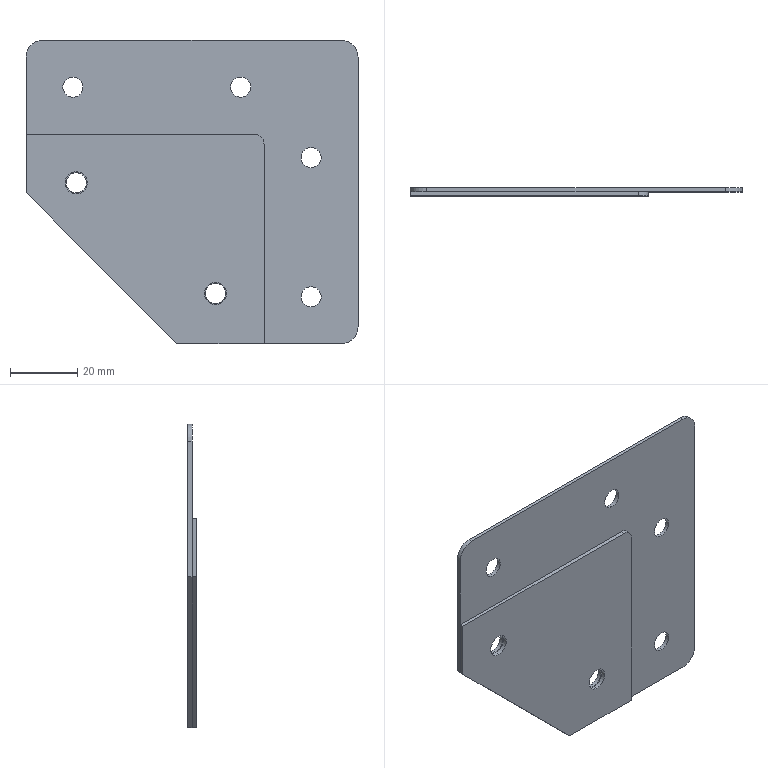Part | SolidWorks | features ICE 9, EdgeFlange 2, Fillet 2, HoleWzd 2, FlatPattern 1, SMBaseFlange 1, SheetMetal 1, WeldmentFeature 1 | 2 solids | 34 faces | box 99 x 2.4 x 90.5 mm | volume 13339 mm3 | cylinder 20 | plane 14 | commonest cylinder face diameters 6 x13 6.6 x4 10 x3
STEP:
#1=CARTESIAN_POINT('',(553.,-1.2,256.7));
#2=VERTEX_POINT('',#1);
#3=CARTESIAN_POINT('',(553.,-1.2,263.3));
#4=VERTEX_POINT('',#3);
#5=CARTESIAN_POINT('',(553.,-1.2,260.));
#6=DIRECTION('',(0.,1.,0.));
#7=DIRECTION('',(0.,0.,1.));
#8=AXIS2_PLACEMENT_3D('',#5,#6,#7);
#9=CIRCLE('',#8,3.3);
#10=EDGE_CURVE('',#2,#4,#9,.T.);
#11=ORIENTED_EDGE('',*,*,#10,.F.);
#12=CARTESIAN_POINT('',(553.,0.,256.7));
#13=VERTEX_POINT('',#12);
#14=CARTESIAN_POINT('',(553.,0.,256.7));
#15=DIRECTION('',(0.,1.,0.));
#16=VECTOR('',#15,1000.);
#17=LINE('',#14,#16);
#18=EDGE_CURVE('',#2,#13,#17,.T.);
#19=ORIENTED_EDGE('',*,*,#18,.T.);
#20=CARTESIAN_POINT('',(553.,0.,263.3));
#21=VERTEX_POINT('',#20);
#22=CARTESIAN_POINT('',(553.,0.,260.));
#23=DIRECTION('',(0.,1.,0.));
#24=DIRECTION('',(0.,0.,1.));
#25=AXIS2_PLACEMENT_3D('',#22,#23,#24);
#26=CIRCLE('',#25,3.3);
#27=EDGE_CURVE('',#13,#21,#26,.T.);
#28=ORIENTED_EDGE('',*,*,#27,.T.);
#29=CARTESIAN_POINT('',(553.,0.,263.3));
#30=DIRECTION('',(0.,1.,0.));
#31=VECTOR('',#30,1000.);
#32=LINE('',#29,#31);
#33=EDGE_CURVE('',#4,#21,#32,.T.);
#34=ORIENTED_EDGE('',*,*,#33,.F.);
#35=EDGE_LOOP('',(#11,#19,#28,#34));
#36=FACE_OUTER_BOUND('',#35,.T.);
#37=CARTESIAN_POINT('',(553.,0.,260.));
#38=DIRECTION('',(0.,1.,0.));
#39=DIRECTION('',(0.,0.,1.));
#40=AXIS2_PLACEMENT_3D('',#37,#38,#39);
#41=CYLINDRICAL_SURFACE('',#40,3.3);
#42=ADVANCED_FACE('',(#36),#41,.F.);
#43=CARTESIAN_POINT('',(511.5,-1.2,289.7));
#44=VERTEX_POINT('',#43);
#45=CARTESIAN_POINT('',(511.5,-1.2,296.3));
#46=VERTEX_POINT('',#45);
#47=CARTESIAN_POINT('',(511.5,-1.2,293.));
#48=DIRECTION('',(0.,1.,0.));
#49=DIRECTION('',(0.,0.,1.));
#50=AXIS2_PLACEMENT_3D('',#47,#48,#49);
#51=CIRCLE('',#50,3.3);
#52=EDGE_CURVE('',#44,#46,#51,.T.);
#53=ORIENTED_EDGE('',*,*,#52,.F.);
#54=CARTESIAN_POINT('',(511.5,0.,289.7));
#55=VERTEX_POINT('',#54);
#56=CARTESIAN_POINT('',(511.5,0.,289.7));
#57=DIRECTION('',(0.,1.,0.));
#58=VECTOR('',#57,1000.);
#59=LINE('',#56,#58);
#60=EDGE_CURVE('',#44,#55,#59,.T.);
#61=ORIENTED_EDGE('',*,*,#60,.T.);
#62=CARTESIAN_POINT('',(511.5,0.,296.3));
#63=VERTEX_POINT('',#62);
#64=CARTESIAN_POINT('',(511.5,0.,293.));
#65=DIRECTION('',(0.,1.,0.));
#66=DIRECTION('',(0.,0.,1.));
#67=AXIS2_PLACEMENT_3D('',#64,#65,#66);
#68=CIRCLE('',#67,3.3);
#69=EDGE_CURVE('',#55,#63,#68,.T.);
#70=ORIENTED_EDGE('',*,*,#69,.T.);
#71=CARTESIAN_POINT('',(511.5,0.,296.3));
#72=DIRECTION('',(0.,1.,0.));
#73=VECTOR('',#72,1000.);
#74=LINE('',#71,#73);
#75=EDGE_CURVE('',#46,#63,#74,.T.);
#76=ORIENTED_EDGE('',*,*,#75,.F.);
#77=EDGE_LOOP('',(#53,#61,#70,#76));
#78=FACE_OUTER_BOUND('',#77,.T.);
#79=CARTESIAN_POINT('',(511.5,0.,293.));
#80=DIRECTION('',(0.,1.,0.));
#81=DIRECTION('',(0.,0.,1.));
#82=AXIS2_PLACEMENT_3D('',#79,#80,#81);
#83=CYLINDRICAL_SURFACE('',#82,3.3);
#84=ADVANCED_FACE('',(#78),#83,.F.);
#85=CARTESIAN_POINT('',(567.5,-1.2,304.5));
#86=VERTEX_POINT('',#85);
#87=CARTESIAN_POINT('',(567.5,-1.2,245.));
#88=VERTEX_POINT('',#87);
#89=CARTESIAN_POINT('',(567.5,-1.2,-307.5));
#90=DIRECTION('',(0.,0.,-1.));
#91=VECTOR('',#90,1000.);
#92=LINE('',#89,#91);
#93=EDGE_CURVE('',#86,#88,#92,.T.);
#94=ORIENTED_EDGE('',*,*,#93,.T.);
#95=CARTESIAN_POINT('',(567.5,0.,245.));
#96=VERTEX_POINT('',#95);
#97=CARTESIAN_POINT('',(567.5,-1.2,245.));
#98=DIRECTION('',(0.,1.,0.));
#99=VECTOR('',#98,1000.);
#100=LINE('',#97,#99);
#101=EDGE_CURVE('',#88,#96,#100,.T.);
#102=ORIENTED_EDGE('',*,*,#101,.T.);
#103=CARTESIAN_POINT('',(567.5,0.,304.5));
#104=VERTEX_POINT('',#103);
#105=CARTESIAN_POINT('',(567.5,0.,-307.5));
#106=DIRECTION('',(0.,0.,-1.));
#107=VECTOR('',#106,1000.);
#108=LINE('',#105,#107);
#109=EDGE_CURVE('',#104,#96,#108,.T.);
#110=ORIENTED_EDGE('',*,*,#109,.F.);
#111=CARTESIAN_POINT('',(567.5,-1.2,304.5));
#112=DIRECTION('',(0.,-1.,0.));
#113=VECTOR('',#112,1000.);
#114=LINE('',#111,#113);
#115=EDGE_CURVE('',#104,#86,#114,.T.);
#116=ORIENTED_EDGE('',*,*,#115,.T.);
#117=EDGE_LOOP('',(#94,#102,#110,#116));
#118=FACE_OUTER_BOUND('',#117,.T.);
#119=CARTESIAN_POINT('',(567.5,-1.2,-307.5));
#120=DIRECTION('',(1.,0.,0.));
#121=DIRECTION('',(0.,0.,-1.));
#122=AXIS2_PLACEMENT_3D('',#119,#120,#121);
#123=PLANE('',#122);
#124=ADVANCED_FACE('',(#118),#123,.T.);
#125=CARTESIAN_POINT('',(496.5,0.,307.5));
#126=VERTEX_POINT('',#125);
#127=CARTESIAN_POINT('',(564.5,0.,307.5));
#128=VERTEX_POINT('',#127);
#129=CARTESIAN_POINT('',(-567.5,0.,307.5));
#130=DIRECTION('',(1.,0.,0.));
#131=VECTOR('',#130,1000.);
#132=LINE('',#129,#131);
#133=EDGE_CURVE('',#126,#128,#132,.T.);
#134=ORIENTED_EDGE('',*,*,#133,.F.);
#135=CARTESIAN_POINT('',(496.5,-1.2,307.5));
#136=VERTEX_POINT('',#135);
#137=CARTESIAN_POINT('',(496.5,-1.2,307.5));
#138=DIRECTION('',(0.,-1.,0.));
#139=VECTOR('',#138,1000.);
#140=LINE('',#137,#139);
#141=EDGE_CURVE('',#126,#136,#140,.T.);
#142=ORIENTED_EDGE('',*,*,#141,.T.);
#143=CARTESIAN_POINT('',(564.5,-1.2,307.5));
#144=VERTEX_POINT('',#143);
#145=CARTESIAN_POINT('',(-567.5,-1.2,307.5));
#146=DIRECTION('',(1.,0.,0.));
#147=VECTOR('',#146,1000.);
#148=LINE('',#145,#147);
#149=EDGE_CURVE('',#136,#144,#148,.T.);
#150=ORIENTED_EDGE('',*,*,#149,.T.);
#151=CARTESIAN_POINT('',(564.5,-1.2,307.5));
#152=DIRECTION('',(0.,1.,0.));
#153=VECTOR('',#152,1000.);
#154=LINE('',#151,#153);
#155=EDGE_CURVE('',#144,#128,#154,.T.);
#156=ORIENTED_EDGE('',*,*,#155,.T.);
#157=EDGE_LOOP('',(#134,#142,#150,#156));
#158=FACE_OUTER_BOUND('',#157,.T.);
#159=CARTESIAN_POINT('',(-567.5,-1.2,307.5));
#160=DIRECTION('',(0.,0.,1.));
#161=DIRECTION('',(1.,0.,0.));
#162=AXIS2_PLACEMENT_3D('',#159,#160,#161);
#163=PLANE('',#162);
#164=ADVANCED_FACE('',(#158),#163,.T.);
#165=CARTESIAN_POINT('',(511.5,-1.2,293.));
#166=DIRECTION('',(0.,1.,0.));
#167=DIRECTION('',(0.,0.,1.));
#168=AXIS2_PLACEMENT_3D('',#165,#166,#167);
#169=CIRCLE('',#168,3.3);
#170=EDGE_CURVE('',#46,#44,#169,.T.);
#171=ORIENTED_EDGE('',*,*,#170,.T.);
#172=ORIENTED_EDGE('',*,*,#52,.T.);
#173=EDGE_LOOP('',(#171,#172));
#174=FACE_BOUND('',#173,.T.);
#175=CARTESIAN_POINT('',(553.,-1.2,260.));
#176=DIRECTION('',(0.,1.,0.));
#177=DIRECTION('',(0.,0.,1.));
#178=AXIS2_PLACEMENT_3D('',#175,#176,#177);
#179=CIRCLE('',#178,3.3);
#180=EDGE_CURVE('',#4,#2,#179,.T.);
#181=ORIENTED_EDGE('',*,*,#180,.T.);
#182=ORIENTED_EDGE('',*,*,#10,.T.);
#183=EDGE_LOOP('',(#181,#182));
#184=FACE_BOUND('',#183,.T.);
#185=CARTESIAN_POINT('',(496.5,-1.2,290.));
#186=VERTEX_POINT('',#185);
#187=CARTESIAN_POINT('',(496.5,-1.2,0.));
#188=DIRECTION('',(0.,0.,1.));
#189=VECTOR('',#188,1000.);
#190=LINE('',#187,#189);
#191=EDGE_CURVE('',#186,#136,#190,.T.);
#192=ORIENTED_EDGE('',*,*,#191,.F.);
#193=CARTESIAN_POINT('',(541.5,-1.2,245.));
#194=VERTEX_POINT('',#193);
#195=CARTESIAN_POINT('',(393.25,-1.2,393.25));
#196=DIRECTION('',(0.7071,0.,-0.7071));
#197=VECTOR('',#196,1000.);
#198=LINE('',#195,#197);
#199=EDGE_CURVE('',#186,#194,#198,.T.);
#200=ORIENTED_EDGE('',*,*,#199,.T.);
#201=CARTESIAN_POINT('',(0.,-1.2,245.));
#202=DIRECTION('',(-1.,0.,0.));
#203=VECTOR('',#202,1000.);
#204=LINE('',#201,#203);
#205=EDGE_CURVE('',#88,#194,#204,.T.);
#206=ORIENTED_EDGE('',*,*,#205,.F.);
#207=ORIENTED_EDGE('',*,*,#93,.F.);
#208=CARTESIAN_POINT('',(564.5,-1.2,304.5));
#209=DIRECTION('',(0.,-1.,0.));
#210=DIRECTION('',(0.,0.,1.));
#211=AXIS2_PLACEMENT_3D('',#208,#209,#210);
#212=CIRCLE('',#211,3.);
#213=EDGE_CURVE('',#86,#144,#212,.T.);
#214=ORIENTED_EDGE('',*,*,#213,.T.);
#215=ORIENTED_EDGE('',*,*,#149,.F.);
#216=EDGE_LOOP('',(#192,#200,#206,#207,#214,#215));
#217=FACE_OUTER_BOUND('',#216,.T.);
#218=CARTESIAN_POINT('',(0.,-1.2,0.));
#219=DIRECTION('',(0.,1.,0.));
#220=DIRECTION('',(0.,0.,1.));
#221=AXIS2_PLACEMENT_3D('',#218,#219,#220);
#222=PLANE('',#221);
#223=ADVANCED_FACE('',(#174,#184,#217),#222,.F.);
#224=CARTESIAN_POINT('',(496.5,0.,290.));
#225=VERTEX_POINT('',#224);
#226=CARTESIAN_POINT('',(541.5,0.,245.));
#227=VERTEX_POINT('',#226);
#228=CARTESIAN_POINT('',(393.25,0.,393.25));
#229=DIRECTION('',(0.7071,0.,-0.7071));
#230=VECTOR('',#229,1000.);
#231=LINE('',#228,#230);
#232=EDGE_CURVE('',#225,#227,#231,.T.);
#233=ORIENTED_EDGE('',*,*,#232,.F.);
#234=CARTESIAN_POINT('',(496.5,0.,245.));
#235=DIRECTION('',(0.,0.,1.));
#236=VECTOR('',#235,1000.);
#237=LINE('',#234,#236);
#238=EDGE_CURVE('',#225,#126,#237,.T.);
#239=ORIENTED_EDGE('',*,*,#238,.T.);
#240=ORIENTED_EDGE('',*,*,#133,.T.);
#241=CARTESIAN_POINT('',(564.5,0.,304.5));
#242=DIRECTION('',(0.,1.,0.));
#243=DIRECTION('',(0.,0.,1.));
#244=AXIS2_PLACEMENT_3D('',#241,#242,#243);
#245=CIRCLE('',#244,3.);
#246=EDGE_CURVE('',#128,#104,#245,.T.);
#247=ORIENTED_EDGE('',*,*,#246,.T.);
#248=ORIENTED_EDGE('',*,*,#109,.T.);
#249=CARTESIAN_POINT('',(496.5,0.,245.));
#250=DIRECTION('',(-1.,0.,0.));
#251=VECTOR('',#250,1000.);
#252=LINE('',#249,#251);
#253=EDGE_CURVE('',#96,#227,#252,.T.);
#254=ORIENTED_EDGE('',*,*,#253,.T.);
#255=EDGE_LOOP('',(#233,#239,#240,#247,#248,#254));
#256=FACE_OUTER_BOUND('',#255,.T.);
#257=CARTESIAN_POINT('',(511.5,0.,293.));
#258=DIRECTION('',(0.,1.,0.));
#259=DIRECTION('',(0.,0.,1.));
#260=AXIS2_PLACEMENT_3D('',#257,#258,#259);
#261=CIRCLE('',#260,3.3);
#262=EDGE_CURVE('',#63,#55,#261,.T.);
#263=ORIENTED_EDGE('',*,*,#262,.F.);
#264=ORIENTED_EDGE('',*,*,#69,.F.);
#265=EDGE_LOOP('',(#263,#264));
#266=FACE_BOUND('',#265,.T.);
#267=CARTESIAN_POINT('',(553.,0.,260.));
#268=DIRECTION('',(0.,1.,0.));
#269=DIRECTION('',(0.,0.,1.));
#270=AXIS2_PLACEMENT_3D('',#267,#268,#269);
#271=CIRCLE('',#270,3.3);
#272=EDGE_CURVE('',#21,#13,#271,.T.);
#273=ORIENTED_EDGE('',*,*,#272,.F.);
#274=ORIENTED_EDGE('',*,*,#27,.F.);
#275=EDGE_LOOP('',(#273,#274));
#276=FACE_BOUND('',#275,.T.);
#277=CARTESIAN_POINT('',(0.,0.,0.));
#278=DIRECTION('',(0.,1.,0.));
#279=DIRECTION('',(0.,0.,1.));
#280=AXIS2_PLACEMENT_3D('',#277,#278,#279);
#281=PLANE('',#280);
#282=ADVANCED_FACE('',(#256,#266,#276),#281,.T.);
#283=ORIENTED_EDGE('',*,*,#60,.F.);
#284=ORIENTED_EDGE('',*,*,#170,.F.);
#285=ORIENTED_EDGE('',*,*,#75,.T.);
#286=ORIENTED_EDGE('',*,*,#262,.T.);
#287=EDGE_LOOP('',(#283,#284,#285,#286));
#288=FACE_OUTER_BOUND('',#287,.T.);
#289=CARTESIAN_POINT('',(511.5,0.,293.));
#290=DIRECTION('',(0.,1.,0.));
#291=DIRECTION('',(0.,0.,1.));
#292=AXIS2_PLACEMENT_3D('',#289,#290,#291);
#293=CYLINDRICAL_SURFACE('',#292,3.3);
#294=ADVANCED_FACE('',(#288),#293,.F.);
#295=ORIENTED_EDGE('',*,*,#18,.F.);
#296=ORIENTED_EDGE('',*,*,#180,.F.);
#297=ORIENTED_EDGE('',*,*,#33,.T.);
#298=ORIENTED_EDGE('',*,*,#272,.T.);
#299=EDGE_LOOP('',(#295,#296,#297,#298));
#300=FACE_OUTER_BOUND('',#299,.T.);
#301=CARTESIAN_POINT('',(553.,0.,260.));
#302=DIRECTION('',(0.,1.,0.));
#303=DIRECTION('',(0.,0.,1.));
#304=AXIS2_PLACEMENT_3D('',#301,#302,#303);
#305=CYLINDRICAL_SURFACE('',#304,3.3);
#306=ADVANCED_FACE('',(#300),#305,.F.);
#307=ORIENTED_EDGE('',*,*,#213,.F.);
#308=ORIENTED_EDGE('',*,*,#115,.F.);
#309=ORIENTED_EDGE('',*,*,#246,.F.);
#310=ORIENTED_EDGE('',*,*,#155,.F.);
#311=EDGE_LOOP('',(#307,#308,#309,#310));
#312=FACE_OUTER_BOUND('',#311,.T.);
#313=CARTESIAN_POINT('',(564.5,-1.2,304.5));
#314=DIRECTION('',(0.,1.,0.));
#315=DIRECTION('',(0.,0.,1.));
#316=AXIS2_PLACEMENT_3D('',#313,#314,#315);
#317=CYLINDRICAL_SURFACE('',#316,3.);
#318=ADVANCED_FACE('',(#312),#317,.T.);
#319=CARTESIAN_POINT('',(496.5,-8.8,290.));
#320=DIRECTION('',(0.,1.,0.));
#321=VECTOR('',#320,1000.);
#322=LINE('',#319,#321);
#323=EDGE_CURVE('',#186,#225,#322,.T.);
#324=ORIENTED_EDGE('',*,*,#323,.F.);
#325=ORIENTED_EDGE('',*,*,#191,.T.);
#326=ORIENTED_EDGE('',*,*,#141,.F.);
#327=ORIENTED_EDGE('',*,*,#238,.F.);
#328=EDGE_LOOP('',(#324,#325,#326,#327));
#329=FACE_OUTER_BOUND('',#328,.T.);
#330=CARTESIAN_POINT('',(496.5,-10.,245.));
#331=DIRECTION('',(-1.,0.,0.));
#332=DIRECTION('',(0.,0.,1.));
#333=AXIS2_PLACEMENT_3D('',#330,#331,#332);
#334=PLANE('',#333);
#335=ADVANCED_FACE('',(#329),#334,.T.);
#336=CARTESIAN_POINT('',(541.5,-10.,245.));
#337=DIRECTION('',(0.,-1.,0.));
#338=VECTOR('',#337,1000.);
#339=LINE('',#336,#338);
#340=EDGE_CURVE('',#227,#194,#339,.T.);
#341=ORIENTED_EDGE('',*,*,#340,.F.);
#342=ORIENTED_EDGE('',*,*,#253,.F.);
#343=ORIENTED_EDGE('',*,*,#101,.F.);
#344=ORIENTED_EDGE('',*,*,#205,.T.);
#345=EDGE_LOOP('',(#341,#342,#343,#344));
#346=FACE_OUTER_BOUND('',#345,.T.);
#347=CARTESIAN_POINT('',(496.5,-10.,245.));
#348=DIRECTION('',(0.,0.,-1.));
#349=DIRECTION('',(-1.,0.,0.));
#350=AXIS2_PLACEMENT_3D('',#347,#348,#349);
#351=PLANE('',#350);
#352=ADVANCED_FACE('',(#346),#351,.T.);
#353=ORIENTED_EDGE('',*,*,#323,.T.);
#354=ORIENTED_EDGE('',*,*,#232,.T.);
#355=ORIENTED_EDGE('',*,*,#340,.T.);
#356=ORIENTED_EDGE('',*,*,#199,.F.);
#357=EDGE_LOOP('',(#353,#354,#355,#356));
#358=FACE_OUTER_BOUND('',#357,.T.);
#359=CARTESIAN_POINT('',(541.5,-8.8,245.));
#360=DIRECTION('',(0.7071,0.,0.7071));
#361=DIRECTION('',(0.7071,0.,-0.7071));
#362=AXIS2_PLACEMENT_3D('',#359,#360,#361);
#363=PLANE('',#362);
#364=ADVANCED_FACE('',(#358),#363,.F.);
#365=CLOSED_SHELL('',(#42,#84,#124,#164,#223,#282,#294,#306,#318,#335,#352,#364));
#366=MANIFOLD_SOLID_BREP('',#365);
#367=CARTESIAN_POINT('',(560.5,0.,318.5));
#368=VERTEX_POINT('',#367);
#369=CARTESIAN_POINT('',(560.5,0.,324.5));
#370=VERTEX_POINT('',#369);
#371=CARTESIAN_POINT('',(560.5,0.,321.5));
#372=DIRECTION('',(0.,1.,0.));
#373=DIRECTION('',(0.,0.,1.));
#374=AXIS2_PLACEMENT_3D('',#371,#372,#373);
#375=CIRCLE('',#374,3.);
#376=EDGE_CURVE('',#368,#370,#375,.T.);
#377=ORIENTED_EDGE('',*,*,#376,.F.);
#378=CARTESIAN_POINT('',(560.5,1.2,318.5));
#379=VERTEX_POINT('',#378);
#380=CARTESIAN_POINT('',(560.5,-8.8,318.5));
#381=DIRECTION('',(0.,1.,0.));
#382=VECTOR('',#381,1000.);
#383=LINE('',#380,#382);
#384=EDGE_CURVE('',#368,#379,#383,.T.);
#385=ORIENTED_EDGE('',*,*,#384,.T.);
#386=CARTESIAN_POINT('',(560.5,1.2,324.5));
#387=VERTEX_POINT('',#386);
#388=CARTESIAN_POINT('',(560.5,1.2,321.5));
#389=DIRECTION('',(0.,1.,0.));
#390=DIRECTION('',(0.,0.,1.));
#391=AXIS2_PLACEMENT_3D('',#388,#389,#390);
#392=CIRCLE('',#391,3.);
#393=EDGE_CURVE('',#379,#387,#392,.T.);
#394=ORIENTED_EDGE('',*,*,#393,.T.);
#395=CARTESIAN_POINT('',(560.5,-8.8,324.5));
#396=DIRECTION('',(0.,1.,0.));
#397=VECTOR('',#396,1000.);
#398=LINE('',#395,#397);
#399=EDGE_CURVE('',#370,#387,#398,.T.);
#400=ORIENTED_EDGE('',*,*,#399,.F.);
#401=EDGE_LOOP('',(#377,#385,#394,#400));
#402=FACE_OUTER_BOUND('',#401,.T.);
#403=CARTESIAN_POINT('',(560.5,-8.8,321.5));
#404=DIRECTION('',(0.,1.,0.));
#405=DIRECTION('',(0.,0.,1.));
#406=AXIS2_PLACEMENT_3D('',#403,#404,#405);
#407=CYLINDRICAL_SURFACE('',#406,3.);
#408=ADVANCED_FACE('',(#402),#407,.F.);
#409=CARTESIAN_POINT('',(581.5,0.,297.5));
#410=VERTEX_POINT('',#409);
#411=CARTESIAN_POINT('',(581.5,0.,303.5));
#412=VERTEX_POINT('',#411);
#413=CARTESIAN_POINT('',(581.5,0.,300.5));
#414=DIRECTION('',(0.,1.,0.));
#415=DIRECTION('',(0.,0.,1.));
#416=AXIS2_PLACEMENT_3D('',#413,#414,#415);
#417=CIRCLE('',#416,3.);
#418=EDGE_CURVE('',#410,#412,#417,.T.);
#419=ORIENTED_EDGE('',*,*,#418,.F.);
#420=CARTESIAN_POINT('',(581.5,1.2,297.5));
#421=VERTEX_POINT('',#420);
#422=CARTESIAN_POINT('',(581.5,-8.8,297.5));
#423=DIRECTION('',(0.,1.,0.));
#424=VECTOR('',#423,1000.);
#425=LINE('',#422,#424);
#426=EDGE_CURVE('',#410,#421,#425,.T.);
#427=ORIENTED_EDGE('',*,*,#426,.T.);
#428=CARTESIAN_POINT('',(581.5,1.2,303.5));
#429=VERTEX_POINT('',#428);
#430=CARTESIAN_POINT('',(581.5,1.2,300.5));
#431=DIRECTION('',(0.,1.,0.));
#432=DIRECTION('',(0.,0.,1.));
#433=AXIS2_PLACEMENT_3D('',#430,#431,#432);
#434=CIRCLE('',#433,3.);
#435=EDGE_CURVE('',#421,#429,#434,.T.);
#436=ORIENTED_EDGE('',*,*,#435,.T.);
#437=CARTESIAN_POINT('',(581.5,-8.8,303.5));
#438=DIRECTION('',(0.,1.,0.));
#439=VECTOR('',#438,1000.);
#440=LINE('',#437,#439);
#441=EDGE_CURVE('',#412,#429,#440,.T.);
#442=ORIENTED_EDGE('',*,*,#441,.F.);
#443=EDGE_LOOP('',(#419,#427,#436,#442));
#444=FACE_OUTER_BOUND('',#443,.T.);
#445=CARTESIAN_POINT('',(581.5,-8.8,300.5));
#446=DIRECTION('',(0.,1.,0.));
#447=DIRECTION('',(0.,0.,1.));
#448=AXIS2_PLACEMENT_3D('',#445,#446,#447);
#449=CYLINDRICAL_SURFACE('',#448,3.);
#450=ADVANCED_FACE('',(#444),#449,.F.);
#451=CARTESIAN_POINT('',(553.,1.2,257.));
#452=VERTEX_POINT('',#451);
#453=CARTESIAN_POINT('',(553.,1.2,263.));
#454=VERTEX_POINT('',#453);
#455=CARTESIAN_POINT('',(553.,1.2,260.));
#456=DIRECTION('',(0.,1.,0.));
#457=DIRECTION('',(0.,0.,1.));
#458=AXIS2_PLACEMENT_3D('',#455,#456,#457);
#459=CIRCLE('',#458,3.);
#460=EDGE_CURVE('',#452,#454,#459,.T.);
#461=ORIENTED_EDGE('',*,*,#460,.T.);
#462=CARTESIAN_POINT('',(553.,0.,263.));
#463=VERTEX_POINT('',#462);
#464=CARTESIAN_POINT('',(553.,-1.2,263.));
#465=DIRECTION('',(0.,-1.,0.));
#466=VECTOR('',#465,1000.);
#467=LINE('',#464,#466);
#468=EDGE_CURVE('',#454,#463,#467,.T.);
#469=ORIENTED_EDGE('',*,*,#468,.T.);
#470=CARTESIAN_POINT('',(553.,0.,257.));
#471=VERTEX_POINT('',#470);
#472=CARTESIAN_POINT('',(553.,0.,260.));
#473=DIRECTION('',(0.,1.,0.));
#474=DIRECTION('',(0.,0.,1.));
#475=AXIS2_PLACEMENT_3D('',#472,#473,#474);
#476=CIRCLE('',#475,3.);
#477=EDGE_CURVE('',#471,#463,#476,.T.);
#478=ORIENTED_EDGE('',*,*,#477,.F.);
#479=CARTESIAN_POINT('',(553.,-1.2,257.));
#480=DIRECTION('',(0.,-1.,0.));
#481=VECTOR('',#480,1000.);
#482=LINE('',#479,#481);
#483=EDGE_CURVE('',#452,#471,#482,.T.);
#484=ORIENTED_EDGE('',*,*,#483,.F.);
#485=EDGE_LOOP('',(#461,#469,#478,#484));
#486=FACE_OUTER_BOUND('',#485,.T.);
#487=CARTESIAN_POINT('',(553.,-1.2,260.));
#488=DIRECTION('',(0.,-1.,0.));
#489=DIRECTION('',(0.,0.,-1.));
#490=AXIS2_PLACEMENT_3D('',#487,#488,#489);
#491=CYLINDRICAL_SURFACE('',#490,3.);
#492=ADVANCED_FACE('',(#486),#491,.F.);
#493=CARTESIAN_POINT('',(511.5,1.2,290.));
#494=VERTEX_POINT('',#493);
#495=CARTESIAN_POINT('',(511.5,1.2,296.));
#496=VERTEX_POINT('',#495);
#497=CARTESIAN_POINT('',(511.5,1.2,293.));
#498=DIRECTION('',(0.,1.,0.));
#499=DIRECTION('',(0.,0.,1.));
#500=AXIS2_PLACEMENT_3D('',#497,#498,#499);
#501=CIRCLE('',#500,3.);
#502=EDGE_CURVE('',#494,#496,#501,.T.);
#503=ORIENTED_EDGE('',*,*,#502,.T.);
#504=CARTESIAN_POINT('',(511.5,0.,296.));
#505=VERTEX_POINT('',#504);
#506=CARTESIAN_POINT('',(511.5,-1.2,296.));
#507=DIRECTION('',(0.,-1.,0.));
#508=VECTOR('',#507,1000.);
#509=LINE('',#506,#508);
#510=EDGE_CURVE('',#496,#505,#509,.T.);
#511=ORIENTED_EDGE('',*,*,#510,.T.);
#512=CARTESIAN_POINT('',(511.5,0.,290.));
#513=VERTEX_POINT('',#512);
#514=CARTESIAN_POINT('',(511.5,0.,293.));
#515=DIRECTION('',(0.,1.,0.));
#516=DIRECTION('',(0.,0.,1.));
#517=AXIS2_PLACEMENT_3D('',#514,#515,#516);
#518=CIRCLE('',#517,3.);
#519=EDGE_CURVE('',#513,#505,#518,.T.);
#520=ORIENTED_EDGE('',*,*,#519,.F.);
#521=CARTESIAN_POINT('',(511.5,-1.2,290.));
#522=DIRECTION('',(0.,-1.,0.));
#523=VECTOR('',#522,1000.);
#524=LINE('',#521,#523);
#525=EDGE_CURVE('',#494,#513,#524,.T.);
#526=ORIENTED_EDGE('',*,*,#525,.F.);
#527=EDGE_LOOP('',(#503,#511,#520,#526));
#528=FACE_OUTER_BOUND('',#527,.T.);
#529=CARTESIAN_POINT('',(511.5,-1.2,293.));
#530=DIRECTION('',(0.,-1.,0.));
#531=DIRECTION('',(0.,0.,-1.));
#532=AXIS2_PLACEMENT_3D('',#529,#530,#531);
#533=CYLINDRICAL_SURFACE('',#532,3.);
#534=ADVANCED_FACE('',(#528),#533,.F.);
#535=CARTESIAN_POINT('',(510.5,1.2,324.5));
#536=VERTEX_POINT('',#535);
#537=CARTESIAN_POINT('',(510.5,1.2,318.5));
#538=VERTEX_POINT('',#537);
#539=CARTESIAN_POINT('',(510.5,1.2,321.5));
#540=DIRECTION('',(0.,-1.,0.));
#541=DIRECTION('',(0.,0.,-1.));
#542=AXIS2_PLACEMENT_3D('',#539,#540,#541);
#543=CIRCLE('',#542,3.);
#544=EDGE_CURVE('',#536,#538,#543,.T.);
#545=ORIENTED_EDGE('',*,*,#544,.F.);
#546=CARTESIAN_POINT('',(510.5,0.,324.5));
#547=VERTEX_POINT('',#546);
#548=CARTESIAN_POINT('',(510.5,1.2,324.5));
#549=DIRECTION('',(0.,-1.,0.));
#550=VECTOR('',#549,1000.);
#551=LINE('',#548,#550);
#552=EDGE_CURVE('',#536,#547,#551,.T.);
#553=ORIENTED_EDGE('',*,*,#552,.T.);
#554=CARTESIAN_POINT('',(510.5,0.,318.5));
#555=VERTEX_POINT('',#554);
#556=CARTESIAN_POINT('',(510.5,0.,321.5));
#557=DIRECTION('',(0.,-1.,0.));
#558=DIRECTION('',(0.,0.,-1.));
#559=AXIS2_PLACEMENT_3D('',#556,#557,#558);
#560=CIRCLE('',#559,3.);
#561=EDGE_CURVE('',#547,#555,#560,.T.);
#562=ORIENTED_EDGE('',*,*,#561,.T.);
#563=CARTESIAN_POINT('',(510.5,1.2,318.5));
#564=DIRECTION('',(0.,-1.,0.));
#565=VECTOR('',#564,1000.);
#566=LINE('',#563,#565);
#567=EDGE_CURVE('',#538,#555,#566,.T.);
#568=ORIENTED_EDGE('',*,*,#567,.F.);
#569=EDGE_LOOP('',(#545,#553,#562,#568));
#570=FACE_OUTER_BOUND('',#569,.T.);
#571=CARTESIAN_POINT('',(510.5,1.2,321.5));
#572=DIRECTION('',(0.,-1.,0.));
#573=DIRECTION('',(0.,0.,-1.));
#574=AXIS2_PLACEMENT_3D('',#571,#572,#573);
#575=CYLINDRICAL_SURFACE('',#574,3.);
#576=ADVANCED_FACE('',(#570),#575,.F.);
#577=CARTESIAN_POINT('',(581.5,1.2,262.));
#578=VERTEX_POINT('',#577);
#579=CARTESIAN_POINT('',(581.5,1.2,256.));
#580=VERTEX_POINT('',#579);
#581=CARTESIAN_POINT('',(581.5,1.2,259.));
#582=DIRECTION('',(0.,-1.,0.));
#583=DIRECTION('',(0.,0.,-1.));
#584=AXIS2_PLACEMENT_3D('',#581,#582,#583);
#585=CIRCLE('',#584,3.);
#586=EDGE_CURVE('',#578,#580,#585,.T.);
#587=ORIENTED_EDGE('',*,*,#586,.F.);
#588=CARTESIAN_POINT('',(581.5,0.,262.));
#589=VERTEX_POINT('',#588);
#590=CARTESIAN_POINT('',(581.5,1.2,262.));
#591=DIRECTION('',(0.,-1.,0.));
#592=VECTOR('',#591,1000.);
#593=LINE('',#590,#592);
#594=EDGE_CURVE('',#578,#589,#593,.T.);
#595=ORIENTED_EDGE('',*,*,#594,.T.);
#596=CARTESIAN_POINT('',(581.5,0.,256.));
#597=VERTEX_POINT('',#596);
#598=CARTESIAN_POINT('',(581.5,0.,259.));
#599=DIRECTION('',(0.,-1.,0.));
#600=DIRECTION('',(0.,0.,-1.));
#601=AXIS2_PLACEMENT_3D('',#598,#599,#600);
#602=CIRCLE('',#601,3.);
#603=EDGE_CURVE('',#589,#597,#602,.T.);
#604=ORIENTED_EDGE('',*,*,#603,.T.);
#605=CARTESIAN_POINT('',(581.5,1.2,256.));
#606=DIRECTION('',(0.,-1.,0.));
#607=VECTOR('',#606,1000.);
#608=LINE('',#605,#607);
#609=EDGE_CURVE('',#580,#597,#608,.T.);
#610=ORIENTED_EDGE('',*,*,#609,.F.);
#611=EDGE_LOOP('',(#587,#595,#604,#610));
#612=FACE_OUTER_BOUND('',#611,.T.);
#613=CARTESIAN_POINT('',(581.5,1.2,259.));
#614=DIRECTION('',(0.,-1.,0.));
#615=DIRECTION('',(0.,0.,-1.));
#616=AXIS2_PLACEMENT_3D('',#613,#614,#615);
#617=CYLINDRICAL_SURFACE('',#616,3.);
#618=ADVANCED_FACE('',(#612),#617,.F.);
#619=CARTESIAN_POINT('',(496.5,1.2,290.));
#620=VERTEX_POINT('',#619);
#621=CARTESIAN_POINT('',(496.5,1.2,330.5));
#622=VERTEX_POINT('',#621);
#623=CARTESIAN_POINT('',(496.5,1.2,245.));
#624=DIRECTION('',(0.,0.,1.));
#625=VECTOR('',#624,1000.);
#626=LINE('',#623,#625);
#627=EDGE_CURVE('',#620,#622,#626,.T.);
#628=ORIENTED_EDGE('',*,*,#627,.F.);
#629=CARTESIAN_POINT('',(496.5,0.,290.));
#630=VERTEX_POINT('',#629);
#631=CARTESIAN_POINT('',(496.5,-8.8,290.));
#632=DIRECTION('',(0.,1.,0.));
#633=VECTOR('',#632,1000.);
#634=LINE('',#631,#633);
#635=EDGE_CURVE('',#630,#620,#634,.T.);
#636=ORIENTED_EDGE('',*,*,#635,.F.);
#637=CARTESIAN_POINT('',(496.5,0.,330.5));
#638=VERTEX_POINT('',#637);
#639=CARTESIAN_POINT('',(496.5,0.,245.));
#640=DIRECTION('',(0.,0.,1.));
#641=VECTOR('',#640,1000.);
#642=LINE('',#639,#641);
#643=EDGE_CURVE('',#630,#638,#642,.T.);
#644=ORIENTED_EDGE('',*,*,#643,.T.);
#645=CARTESIAN_POINT('',(496.5,1.2,330.5));
#646=DIRECTION('',(0.,1.,0.));
#647=VECTOR('',#646,1000.);
#648=LINE('',#645,#647);
#649=EDGE_CURVE('',#638,#622,#648,.T.);
#650=ORIENTED_EDGE('',*,*,#649,.T.);
#651=EDGE_LOOP('',(#628,#636,#644,#650));
#652=FACE_OUTER_BOUND('',#651,.T.);
#653=CARTESIAN_POINT('',(496.5,1.2,245.));
#654=DIRECTION('',(1.,0.,0.));
#655=DIRECTION('',(0.,0.,-1.));
#656=AXIS2_PLACEMENT_3D('',#653,#654,#655);
#657=PLANE('',#656);
#658=ADVANCED_FACE('',(#652),#657,.F.);
#659=CARTESIAN_POINT('',(501.5,0.,335.5));
#660=VERTEX_POINT('',#659);
#661=CARTESIAN_POINT('',(590.5,0.,335.5));
#662=VERTEX_POINT('',#661);
#663=CARTESIAN_POINT('',(496.5,0.,335.5));
#664=DIRECTION('',(1.,0.,0.));
#665=VECTOR('',#664,1000.);
#666=LINE('',#663,#665);
#667=EDGE_CURVE('',#660,#662,#666,.T.);
#668=ORIENTED_EDGE('',*,*,#667,.T.);
#669=CARTESIAN_POINT('',(590.5,1.2,335.5));
#670=VERTEX_POINT('',#669);
#671=CARTESIAN_POINT('',(590.5,1.2,335.5));
#672=DIRECTION('',(0.,1.,0.));
#673=VECTOR('',#672,1000.);
#674=LINE('',#671,#673);
#675=EDGE_CURVE('',#662,#670,#674,.T.);
#676=ORIENTED_EDGE('',*,*,#675,.T.);
#677=CARTESIAN_POINT('',(501.5,1.2,335.5));
#678=VERTEX_POINT('',#677);
#679=CARTESIAN_POINT('',(496.5,1.2,335.5));
#680=DIRECTION('',(1.,0.,0.));
#681=VECTOR('',#680,1000.);
#682=LINE('',#679,#681);
#683=EDGE_CURVE('',#678,#670,#682,.T.);
#684=ORIENTED_EDGE('',*,*,#683,.F.);
#685=CARTESIAN_POINT('',(501.5,1.2,335.5));
#686=DIRECTION('',(0.,-1.,0.));
#687=VECTOR('',#686,1000.);
#688=LINE('',#685,#687);
#689=EDGE_CURVE('',#678,#660,#688,.T.);
#690=ORIENTED_EDGE('',*,*,#689,.T.);
#691=EDGE_LOOP('',(#668,#676,#684,#690));
#692=FACE_OUTER_BOUND('',#691,.T.);
#693=CARTESIAN_POINT('',(496.5,1.2,335.5));
#694=DIRECTION('',(0.,0.,-1.));
#695=DIRECTION('',(-1.,0.,0.));
#696=AXIS2_PLACEMENT_3D('',#693,#694,#695);
#697=PLANE('',#696);
#698=ADVANCED_FACE('',(#692),#697,.F.);
#699=CARTESIAN_POINT('',(595.5,0.,330.5));
#700=VERTEX_POINT('',#699);
#701=CARTESIAN_POINT('',(595.5,0.,250.));
#702=VERTEX_POINT('',#701);
#703=CARTESIAN_POINT('',(595.5,0.,245.));
#704=DIRECTION('',(0.,0.,-1.));
#705=VECTOR('',#704,1000.);
#706=LINE('',#703,#705);
#707=EDGE_CURVE('',#700,#702,#706,.T.);
#708=ORIENTED_EDGE('',*,*,#707,.T.);
#709=CARTESIAN_POINT('',(595.5,1.2,250.));
#710=VERTEX_POINT('',#709);
#711=CARTESIAN_POINT('',(595.5,1.2,250.));
#712=DIRECTION('',(0.,1.,0.));
#713=VECTOR('',#712,1000.);
#714=LINE('',#711,#713);
#715=EDGE_CURVE('',#702,#710,#714,.T.);
#716=ORIENTED_EDGE('',*,*,#715,.T.);
#717=CARTESIAN_POINT('',(595.5,1.2,330.5));
#718=VERTEX_POINT('',#717);
#719=CARTESIAN_POINT('',(595.5,1.2,245.));
#720=DIRECTION('',(0.,0.,-1.));
#721=VECTOR('',#720,1000.);
#722=LINE('',#719,#721);
#723=EDGE_CURVE('',#718,#710,#722,.T.);
#724=ORIENTED_EDGE('',*,*,#723,.F.);
#725=CARTESIAN_POINT('',(595.5,1.2,330.5));
#726=DIRECTION('',(0.,-1.,0.));
#727=VECTOR('',#726,1000.);
#728=LINE('',#725,#727);
#729=EDGE_CURVE('',#718,#700,#728,.T.);
#730=ORIENTED_EDGE('',*,*,#729,.T.);
#731=EDGE_LOOP('',(#708,#716,#724,#730));
#732=FACE_OUTER_BOUND('',#731,.T.);
#733=CARTESIAN_POINT('',(595.5,1.2,245.));
#734=DIRECTION('',(-1.,0.,0.));
#735=DIRECTION('',(0.,0.,1.));
#736=AXIS2_PLACEMENT_3D('',#733,#734,#735);
#737=PLANE('',#736);
#738=ADVANCED_FACE('',(#732),#737,.F.);
#739=CARTESIAN_POINT('',(590.5,0.,245.));
#740=VERTEX_POINT('',#739);
#741=CARTESIAN_POINT('',(541.5,0.,245.));
#742=VERTEX_POINT('',#741);
#743=CARTESIAN_POINT('',(496.5,0.,245.));
#744=DIRECTION('',(-1.,0.,0.));
#745=VECTOR('',#744,1000.);
#746=LINE('',#743,#745);
#747=EDGE_CURVE('',#740,#742,#746,.T.);
#748=ORIENTED_EDGE('',*,*,#747,.T.);
#749=CARTESIAN_POINT('',(541.5,1.2,245.));
#750=VERTEX_POINT('',#749);
#751=CARTESIAN_POINT('',(541.5,-8.8,245.));
#752=DIRECTION('',(0.,1.,0.));
#753=VECTOR('',#752,1000.);
#754=LINE('',#751,#753);
#755=EDGE_CURVE('',#742,#750,#754,.T.);
#756=ORIENTED_EDGE('',*,*,#755,.T.);
#757=CARTESIAN_POINT('',(590.5,1.2,245.));
#758=VERTEX_POINT('',#757);
#759=CARTESIAN_POINT('',(496.5,1.2,245.));
#760=DIRECTION('',(-1.,0.,0.));
#761=VECTOR('',#760,1000.);
#762=LINE('',#759,#761);
#763=EDGE_CURVE('',#758,#750,#762,.T.);
#764=ORIENTED_EDGE('',*,*,#763,.F.);
#765=CARTESIAN_POINT('',(590.5,1.2,245.));
#766=DIRECTION('',(0.,-1.,0.));
#767=VECTOR('',#766,1000.);
#768=LINE('',#765,#767);
#769=EDGE_CURVE('',#758,#740,#768,.T.);
#770=ORIENTED_EDGE('',*,*,#769,.T.);
#771=EDGE_LOOP('',(#748,#756,#764,#770));
#772=FACE_OUTER_BOUND('',#771,.T.);
#773=CARTESIAN_POINT('',(496.5,1.2,245.));
#774=DIRECTION('',(0.,0.,1.));
#775=DIRECTION('',(1.,0.,0.));
#776=AXIS2_PLACEMENT_3D('',#773,#774,#775);
#777=PLANE('',#776);
#778=ADVANCED_FACE('',(#772),#777,.F.);
#779=CARTESIAN_POINT('',(560.5,1.2,321.5));
#780=DIRECTION('',(0.,1.,0.));
#781=DIRECTION('',(0.,0.,1.));
#782=AXIS2_PLACEMENT_3D('',#779,#780,#781);
#783=CIRCLE('',#782,3.);
#784=EDGE_CURVE('',#387,#379,#783,.T.);
#785=ORIENTED_EDGE('',*,*,#784,.F.);
#786=ORIENTED_EDGE('',*,*,#393,.F.);
#787=EDGE_LOOP('',(#785,#786));
#788=FACE_BOUND('',#787,.T.);
#789=CARTESIAN_POINT('',(581.5,1.2,300.5));
#790=DIRECTION('',(0.,1.,0.));
#791=DIRECTION('',(0.,0.,1.));
#792=AXIS2_PLACEMENT_3D('',#789,#790,#791);
#793=CIRCLE('',#792,3.);
#794=EDGE_CURVE('',#429,#421,#793,.T.);
#795=ORIENTED_EDGE('',*,*,#794,.F.);
#796=ORIENTED_EDGE('',*,*,#435,.F.);
#797=EDGE_LOOP('',(#795,#796));
#798=FACE_BOUND('',#797,.T.);
#799=CARTESIAN_POINT('',(541.5,1.2,245.));
#800=DIRECTION('',(0.7071,0.,-0.7071));
#801=VECTOR('',#800,1000.);
#802=LINE('',#799,#801);
#803=EDGE_CURVE('',#620,#750,#802,.T.);
#804=ORIENTED_EDGE('',*,*,#803,.F.);
#805=ORIENTED_EDGE('',*,*,#627,.T.);
#806=CARTESIAN_POINT('',(501.5,1.2,330.5));
#807=DIRECTION('',(0.,1.,0.));
#808=DIRECTION('',(0.,0.,1.));
#809=AXIS2_PLACEMENT_3D('',#806,#807,#808);
#810=CIRCLE('',#809,5.);
#811=EDGE_CURVE('',#622,#678,#810,.T.);
#812=ORIENTED_EDGE('',*,*,#811,.T.);
#813=ORIENTED_EDGE('',*,*,#683,.T.);
#814=CARTESIAN_POINT('',(590.5,1.2,330.5));
#815=DIRECTION('',(0.,1.,0.));
#816=DIRECTION('',(0.,0.,1.));
#817=AXIS2_PLACEMENT_3D('',#814,#815,#816);
#818=CIRCLE('',#817,5.);
#819=EDGE_CURVE('',#670,#718,#818,.T.);
#820=ORIENTED_EDGE('',*,*,#819,.T.);
#821=ORIENTED_EDGE('',*,*,#723,.T.);
#822=CARTESIAN_POINT('',(590.5,1.2,250.));
#823=DIRECTION('',(0.,1.,0.));
#824=DIRECTION('',(0.,0.,1.));
#825=AXIS2_PLACEMENT_3D('',#822,#823,#824);
#826=CIRCLE('',#825,5.);
#827=EDGE_CURVE('',#710,#758,#826,.T.);
#828=ORIENTED_EDGE('',*,*,#827,.T.);
#829=ORIENTED_EDGE('',*,*,#763,.T.);
#830=EDGE_LOOP('',(#804,#805,#812,#813,#820,#821,#828,#829));
#831=FACE_OUTER_BOUND('',#830,.T.);
#832=ORIENTED_EDGE('',*,*,#460,.F.);
#833=CARTESIAN_POINT('',(553.,1.2,260.));
#834=DIRECTION('',(0.,1.,0.));
#835=DIRECTION('',(0.,0.,1.));
#836=AXIS2_PLACEMENT_3D('',#833,#834,#835);
#837=CIRCLE('',#836,3.);
#838=EDGE_CURVE('',#454,#452,#837,.T.);
#839=ORIENTED_EDGE('',*,*,#838,.F.);
#840=EDGE_LOOP('',(#832,#839));
#841=FACE_BOUND('',#840,.T.);
#842=ORIENTED_EDGE('',*,*,#502,.F.);
#843=CARTESIAN_POINT('',(511.5,1.2,293.));
#844=DIRECTION('',(0.,1.,0.));
#845=DIRECTION('',(0.,0.,1.));
#846=AXIS2_PLACEMENT_3D('',#843,#844,#845);
#847=CIRCLE('',#846,3.);
#848=EDGE_CURVE('',#496,#494,#847,.T.);
#849=ORIENTED_EDGE('',*,*,#848,.F.);
#850=EDGE_LOOP('',(#842,#849));
#851=FACE_BOUND('',#850,.T.);
#852=CARTESIAN_POINT('',(510.5,1.2,321.5));
#853=DIRECTION('',(0.,-1.,0.));
#854=DIRECTION('',(0.,0.,-1.));
#855=AXIS2_PLACEMENT_3D('',#852,#853,#854);
#856=CIRCLE('',#855,3.);
#857=EDGE_CURVE('',#538,#536,#856,.T.);
#858=ORIENTED_EDGE('',*,*,#857,.T.);
#859=ORIENTED_EDGE('',*,*,#544,.T.);
#860=EDGE_LOOP('',(#858,#859));
#861=FACE_BOUND('',#860,.T.);
#862=CARTESIAN_POINT('',(581.5,1.2,259.));
#863=DIRECTION('',(0.,-1.,0.));
#864=DIRECTION('',(0.,0.,-1.));
#865=AXIS2_PLACEMENT_3D('',#862,#863,#864);
#866=CIRCLE('',#865,3.);
#867=EDGE_CURVE('',#580,#578,#866,.T.);
#868=ORIENTED_EDGE('',*,*,#867,.T.);
#869=ORIENTED_EDGE('',*,*,#586,.T.);
#870=EDGE_LOOP('',(#868,#869));
#871=FACE_BOUND('',#870,.T.);
#872=CARTESIAN_POINT('',(0.,1.2,0.));
#873=DIRECTION('',(0.,1.,0.));
#874=DIRECTION('',(0.,0.,1.));
#875=AXIS2_PLACEMENT_3D('',#872,#873,#874);
#876=PLANE('',#875);
#877=ADVANCED_FACE('',(#788,#798,#831,#841,#851,#861,#871),#876,.T.);
#878=CARTESIAN_POINT('',(560.5,0.,321.5));
#879=DIRECTION('',(0.,1.,0.));
#880=DIRECTION('',(0.,0.,1.));
#881=AXIS2_PLACEMENT_3D('',#878,#879,#880);
#882=CIRCLE('',#881,3.);
#883=EDGE_CURVE('',#370,#368,#882,.T.);
#884=ORIENTED_EDGE('',*,*,#883,.T.);
#885=ORIENTED_EDGE('',*,*,#376,.T.);
#886=EDGE_LOOP('',(#884,#885));
#887=FACE_BOUND('',#886,.T.);
#888=CARTESIAN_POINT('',(581.5,0.,300.5));
#889=DIRECTION('',(0.,1.,0.));
#890=DIRECTION('',(0.,0.,1.));
#891=AXIS2_PLACEMENT_3D('',#888,#889,#890);
#892=CIRCLE('',#891,3.);
#893=EDGE_CURVE('',#412,#410,#892,.T.);
#894=ORIENTED_EDGE('',*,*,#893,.T.);
#895=ORIENTED_EDGE('',*,*,#418,.T.);
#896=EDGE_LOOP('',(#894,#895));
#897=FACE_BOUND('',#896,.T.);
#898=ORIENTED_EDGE('',*,*,#477,.T.);
#899=CARTESIAN_POINT('',(553.,0.,260.));
#900=DIRECTION('',(0.,1.,0.));
#901=DIRECTION('',(0.,0.,1.));
#902=AXIS2_PLACEMENT_3D('',#899,#900,#901);
#903=CIRCLE('',#902,3.);
#904=EDGE_CURVE('',#463,#471,#903,.T.);
#905=ORIENTED_EDGE('',*,*,#904,.T.);
#906=EDGE_LOOP('',(#898,#905));
#907=FACE_BOUND('',#906,.T.);
#908=ORIENTED_EDGE('',*,*,#519,.T.);
#909=CARTESIAN_POINT('',(511.5,0.,293.));
#910=DIRECTION('',(0.,1.,0.));
#911=DIRECTION('',(0.,0.,1.));
#912=AXIS2_PLACEMENT_3D('',#909,#910,#911);
#913=CIRCLE('',#912,3.);
#914=EDGE_CURVE('',#505,#513,#913,.T.);
#915=ORIENTED_EDGE('',*,*,#914,.T.);
#916=EDGE_LOOP('',(#908,#915));
#917=FACE_BOUND('',#916,.T.);
#918=CARTESIAN_POINT('',(510.5,0.,321.5));
#919=DIRECTION('',(0.,-1.,0.));
#920=DIRECTION('',(0.,0.,-1.));
#921=AXIS2_PLACEMENT_3D('',#918,#919,#920);
#922=CIRCLE('',#921,3.);
#923=EDGE_CURVE('',#555,#547,#922,.T.);
#924=ORIENTED_EDGE('',*,*,#923,.F.);
#925=ORIENTED_EDGE('',*,*,#561,.F.);
#926=EDGE_LOOP('',(#924,#925));
#927=FACE_BOUND('',#926,.T.);
#928=CARTESIAN_POINT('',(581.5,0.,259.));
#929=DIRECTION('',(0.,-1.,0.));
#930=DIRECTION('',(0.,0.,-1.));
#931=AXIS2_PLACEMENT_3D('',#928,#929,#930);
#932=CIRCLE('',#931,3.);
#933=EDGE_CURVE('',#597,#589,#932,.T.);
#934=ORIENTED_EDGE('',*,*,#933,.F.);
#935=ORIENTED_EDGE('',*,*,#603,.F.);
#936=EDGE_LOOP('',(#934,#935));
#937=FACE_BOUND('',#936,.T.);
#938=ORIENTED_EDGE('',*,*,#643,.F.);
#939=CARTESIAN_POINT('',(393.25,0.,393.25));
#940=DIRECTION('',(0.7071,0.,-0.7071));
#941=VECTOR('',#940,1000.);
#942=LINE('',#939,#941);
#943=EDGE_CURVE('',#630,#742,#942,.T.);
#944=ORIENTED_EDGE('',*,*,#943,.T.);
#945=ORIENTED_EDGE('',*,*,#747,.F.);
#946=CARTESIAN_POINT('',(590.5,0.,250.));
#947=DIRECTION('',(0.,-1.,0.));
#948=DIRECTION('',(0.,0.,1.));
#949=AXIS2_PLACEMENT_3D('',#946,#947,#948);
#950=CIRCLE('',#949,5.);
#951=EDGE_CURVE('',#740,#702,#950,.T.);
#952=ORIENTED_EDGE('',*,*,#951,.T.);
#953=ORIENTED_EDGE('',*,*,#707,.F.);
#954=CARTESIAN_POINT('',(590.5,0.,330.5));
#955=DIRECTION('',(0.,-1.,0.));
#956=DIRECTION('',(0.,0.,1.));
#957=AXIS2_PLACEMENT_3D('',#954,#955,#956);
#958=CIRCLE('',#957,5.);
#959=EDGE_CURVE('',#700,#662,#958,.T.);
#960=ORIENTED_EDGE('',*,*,#959,.T.);
#961=ORIENTED_EDGE('',*,*,#667,.F.);
#962=CARTESIAN_POINT('',(501.5,0.,330.5));
#963=DIRECTION('',(0.,-1.,0.));
#964=DIRECTION('',(0.,0.,1.));
#965=AXIS2_PLACEMENT_3D('',#962,#963,#964);
#966=CIRCLE('',#965,5.);
#967=EDGE_CURVE('',#660,#638,#966,.T.);
#968=ORIENTED_EDGE('',*,*,#967,.T.);
#969=EDGE_LOOP('',(#938,#944,#945,#952,#953,#960,#961,#968));
#970=FACE_OUTER_BOUND('',#969,.T.);
#971=CARTESIAN_POINT('',(0.,0.,0.));
#972=DIRECTION('',(0.,1.,0.));
#973=DIRECTION('',(0.,0.,1.));
#974=AXIS2_PLACEMENT_3D('',#971,#972,#973);
#975=PLANE('',#974);
#976=ADVANCED_FACE('',(#887,#897,#907,#917,#927,#937,#970),#975,.F.);
#977=ORIENTED_EDGE('',*,*,#594,.F.);
#978=ORIENTED_EDGE('',*,*,#867,.F.);
#979=ORIENTED_EDGE('',*,*,#609,.T.);
#980=ORIENTED_EDGE('',*,*,#933,.T.);
#981=EDGE_LOOP('',(#977,#978,#979,#980));
#982=FACE_OUTER_BOUND('',#981,.T.);
#983=CARTESIAN_POINT('',(581.5,1.2,259.));
#984=DIRECTION('',(0.,-1.,0.));
#985=DIRECTION('',(0.,0.,-1.));
#986=AXIS2_PLACEMENT_3D('',#983,#984,#985);
#987=CYLINDRICAL_SURFACE('',#986,3.);
#988=ADVANCED_FACE('',(#982),#987,.F.);
#989=ORIENTED_EDGE('',*,*,#552,.F.);
#990=ORIENTED_EDGE('',*,*,#857,.F.);
#991=ORIENTED_EDGE('',*,*,#567,.T.);
#992=ORIENTED_EDGE('',*,*,#923,.T.);
#993=EDGE_LOOP('',(#989,#990,#991,#992));
#994=FACE_OUTER_BOUND('',#993,.T.);
#995=CARTESIAN_POINT('',(510.5,1.2,321.5));
#996=DIRECTION('',(0.,-1.,0.));
#997=DIRECTION('',(0.,0.,-1.));
#998=AXIS2_PLACEMENT_3D('',#995,#996,#997);
#999=CYLINDRICAL_SURFACE('',#998,3.);
#1000=ADVANCED_FACE('',(#994),#999,.F.);
#1001=ORIENTED_EDGE('',*,*,#510,.F.);
#1002=ORIENTED_EDGE('',*,*,#848,.T.);
#1003=ORIENTED_EDGE('',*,*,#525,.T.);
#1004=ORIENTED_EDGE('',*,*,#914,.F.);
#1005=EDGE_LOOP('',(#1001,#1002,#1003,#1004));
#1006=FACE_OUTER_BOUND('',#1005,.T.);
#1007=CARTESIAN_POINT('',(511.5,-1.2,293.));
#1008=DIRECTION('',(0.,-1.,0.));
#1009=DIRECTION('',(0.,0.,-1.));
#1010=AXIS2_PLACEMENT_3D('',#1007,#1008,#1009);
#1011=CYLINDRICAL_SURFACE('',#1010,3.);
#1012=ADVANCED_FACE('',(#1006),#1011,.F.);
#1013=ORIENTED_EDGE('',*,*,#468,.F.);
#1014=ORIENTED_EDGE('',*,*,#838,.T.);
#1015=ORIENTED_EDGE('',*,*,#483,.T.);
#1016=ORIENTED_EDGE('',*,*,#904,.F.);
#1017=EDGE_LOOP('',(#1013,#1014,#1015,#1016));
#1018=FACE_OUTER_BOUND('',#1017,.T.);
#1019=CARTESIAN_POINT('',(553.,-1.2,260.));
#1020=DIRECTION('',(0.,-1.,0.));
#1021=DIRECTION('',(0.,0.,-1.));
#1022=AXIS2_PLACEMENT_3D('',#1019,#1020,#1021);
#1023=CYLINDRICAL_SURFACE('',#1022,3.);
#1024=ADVANCED_FACE('',(#1018),#1023,.F.);
#1025=ORIENTED_EDGE('',*,*,#827,.F.);
#1026=ORIENTED_EDGE('',*,*,#715,.F.);
#1027=ORIENTED_EDGE('',*,*,#951,.F.);
#1028=ORIENTED_EDGE('',*,*,#769,.F.);
#1029=EDGE_LOOP('',(#1025,#1026,#1027,#1028));
#1030=FACE_OUTER_BOUND('',#1029,.T.);
#1031=CARTESIAN_POINT('',(590.5,1.2,250.));
#1032=DIRECTION('',(0.,-1.,0.));
#1033=DIRECTION('',(0.,0.,-1.));
#1034=AXIS2_PLACEMENT_3D('',#1031,#1032,#1033);
#1035=CYLINDRICAL_SURFACE('',#1034,5.);
#1036=ADVANCED_FACE('',(#1030),#1035,.T.);
#1037=ORIENTED_EDGE('',*,*,#819,.F.);
#1038=ORIENTED_EDGE('',*,*,#675,.F.);
#1039=ORIENTED_EDGE('',*,*,#959,.F.);
#1040=ORIENTED_EDGE('',*,*,#729,.F.);
#1041=EDGE_LOOP('',(#1037,#1038,#1039,#1040));
#1042=FACE_OUTER_BOUND('',#1041,.T.);
#1043=CARTESIAN_POINT('',(590.5,1.2,330.5));
#1044=DIRECTION('',(0.,-1.,0.));
#1045=DIRECTION('',(0.,0.,-1.));
#1046=AXIS2_PLACEMENT_3D('',#1043,#1044,#1045);
#1047=CYLINDRICAL_SURFACE('',#1046,5.);
#1048=ADVANCED_FACE('',(#1042),#1047,.T.);
#1049=ORIENTED_EDGE('',*,*,#811,.F.);
#1050=ORIENTED_EDGE('',*,*,#649,.F.);
#1051=ORIENTED_EDGE('',*,*,#967,.F.);
#1052=ORIENTED_EDGE('',*,*,#689,.F.);
#1053=EDGE_LOOP('',(#1049,#1050,#1051,#1052));
#1054=FACE_OUTER_BOUND('',#1053,.T.);
#1055=CARTESIAN_POINT('',(501.5,1.2,330.5));
#1056=DIRECTION('',(0.,-1.,0.));
#1057=DIRECTION('',(0.,0.,-1.));
#1058=AXIS2_PLACEMENT_3D('',#1055,#1056,#1057);
#1059=CYLINDRICAL_SURFACE('',#1058,5.);
#1060=ADVANCED_FACE('',(#1054),#1059,.T.);
#1061=ORIENTED_EDGE('',*,*,#635,.T.);
#1062=ORIENTED_EDGE('',*,*,#803,.T.);
#1063=ORIENTED_EDGE('',*,*,#755,.F.);
#1064=ORIENTED_EDGE('',*,*,#943,.F.);
#1065=EDGE_LOOP('',(#1061,#1062,#1063,#1064));
#1066=FACE_OUTER_BOUND('',#1065,.T.);
#1067=CARTESIAN_POINT('',(541.5,-8.8,245.));
#1068=DIRECTION('',(0.7071,0.,0.7071));
#1069=DIRECTION('',(0.7071,0.,-0.7071));
#1070=AXIS2_PLACEMENT_3D('',#1067,#1068,#1069);
#1071=PLANE('',#1070);
#1072=ADVANCED_FACE('',(#1066),#1071,.F.);
#1073=ORIENTED_EDGE('',*,*,#426,.F.);
#1074=ORIENTED_EDGE('',*,*,#893,.F.);
#1075=ORIENTED_EDGE('',*,*,#441,.T.);
#1076=ORIENTED_EDGE('',*,*,#794,.T.);
#1077=EDGE_LOOP('',(#1073,#1074,#1075,#1076));
#1078=FACE_OUTER_BOUND('',#1077,.T.);
#1079=CARTESIAN_POINT('',(581.5,-8.8,300.5));
#1080=DIRECTION('',(0.,1.,0.));
#1081=DIRECTION('',(0.,0.,1.));
#1082=AXIS2_PLACEMENT_3D('',#1079,#1080,#1081);
#1083=CYLINDRICAL_SURFACE('',#1082,3.);
#1084=ADVANCED_FACE('',(#1078),#1083,.F.);
#1085=ORIENTED_EDGE('',*,*,#384,.F.);
#1086=ORIENTED_EDGE('',*,*,#883,.F.);
#1087=ORIENTED_EDGE('',*,*,#399,.T.);
#1088=ORIENTED_EDGE('',*,*,#784,.T.);
#1089=EDGE_LOOP('',(#1085,#1086,#1087,#1088));
#1090=FACE_OUTER_BOUND('',#1089,.T.);
#1091=CARTESIAN_POINT('',(560.5,-8.8,321.5));
#1092=DIRECTION('',(0.,1.,0.));
#1093=DIRECTION('',(0.,0.,1.));
#1094=AXIS2_PLACEMENT_3D('',#1091,#1092,#1093);
#1095=CYLINDRICAL_SURFACE('',#1094,3.);
#1096=ADVANCED_FACE('',(#1090),#1095,.F.);
#1097=CLOSED_SHELL('',(#408,#450,#492,#534,#576,#618,#658,#698,#738,#778,#877,#976,#988,#1000,#1012,#1024,#1036,#1048,#1060,#1072,#1084,#1096));
#1098=MANIFOLD_SOLID_BREP('',#1097);
#1099=CARTESIAN_POINT('',(0.,0.,0.));
#1100=DIRECTION('',(0.,0.,1.));
#1101=DIRECTION('',(1.,0.,0.));
#1102=AXIS2_PLACEMENT_3D('',#1099,#1100,#1101);
#1103=(LENGTH_UNIT()NAMED_UNIT(*)SI_UNIT(.MILLI.,.METRE.));
#1104=UNCERTAINTY_MEASURE_WITH_UNIT(LENGTH_MEASURE(0.00001),#1103,'','');
#1105=(NAMED_UNIT(*)PLANE_ANGLE_UNIT()SI_UNIT($,.RADIAN.));
#1106=(NAMED_UNIT(*)SI_UNIT($,.STERADIAN.)SOLID_ANGLE_UNIT());
#1107=(GEOMETRIC_REPRESENTATION_CONTEXT(3)GLOBAL_UNCERTAINTY_ASSIGNED_CONTEXT((#1104))GLOBAL_UNIT_ASSIGNED_CONTEXT((#1103,#1105,#1106))REPRESENTATION_CONTEXT('',''));
#1108=ADVANCED_BREP_SHAPE_REPRESENTATION('',(#366,#1098,#1102),#1107);